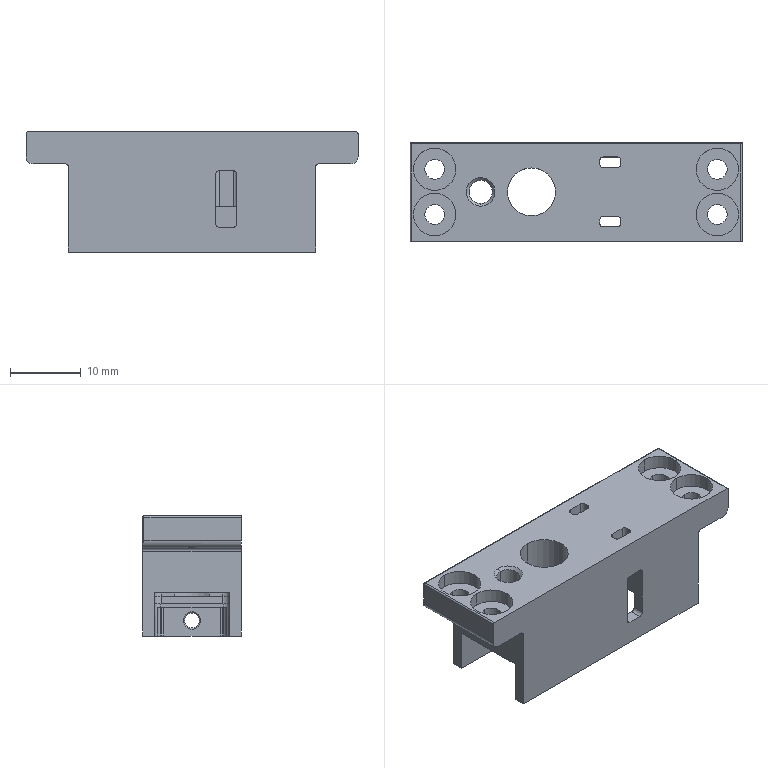NC program | NX | posted with a generic post | part box 47 x 14 x 17 mm
Lines 3150 to 3166 of 3166:
(ZLEVEL_PROFILE_COPY_1_COPY_COPY_COPY_COPY_2_COPY_COPY_COPY , TOOL : D6A45)
N6292 T18 M6
N6294 G54
N6296 G17 G0 G90 X-4.309 Y-2.041 B0. C0. S7000 M3
N6298 G43 Z30. H18
N6300 Z0.
N6302 G94 G1 Z-1. F1000.
N6304 Y4.041
N6306 X-5.391
N6308 Y-2.041
N6310 X-4.309
N6312 G3 X-4.609 Y-1.522 R0.6
N6314 G0 Z30.
N6316 M5
N6318 M2